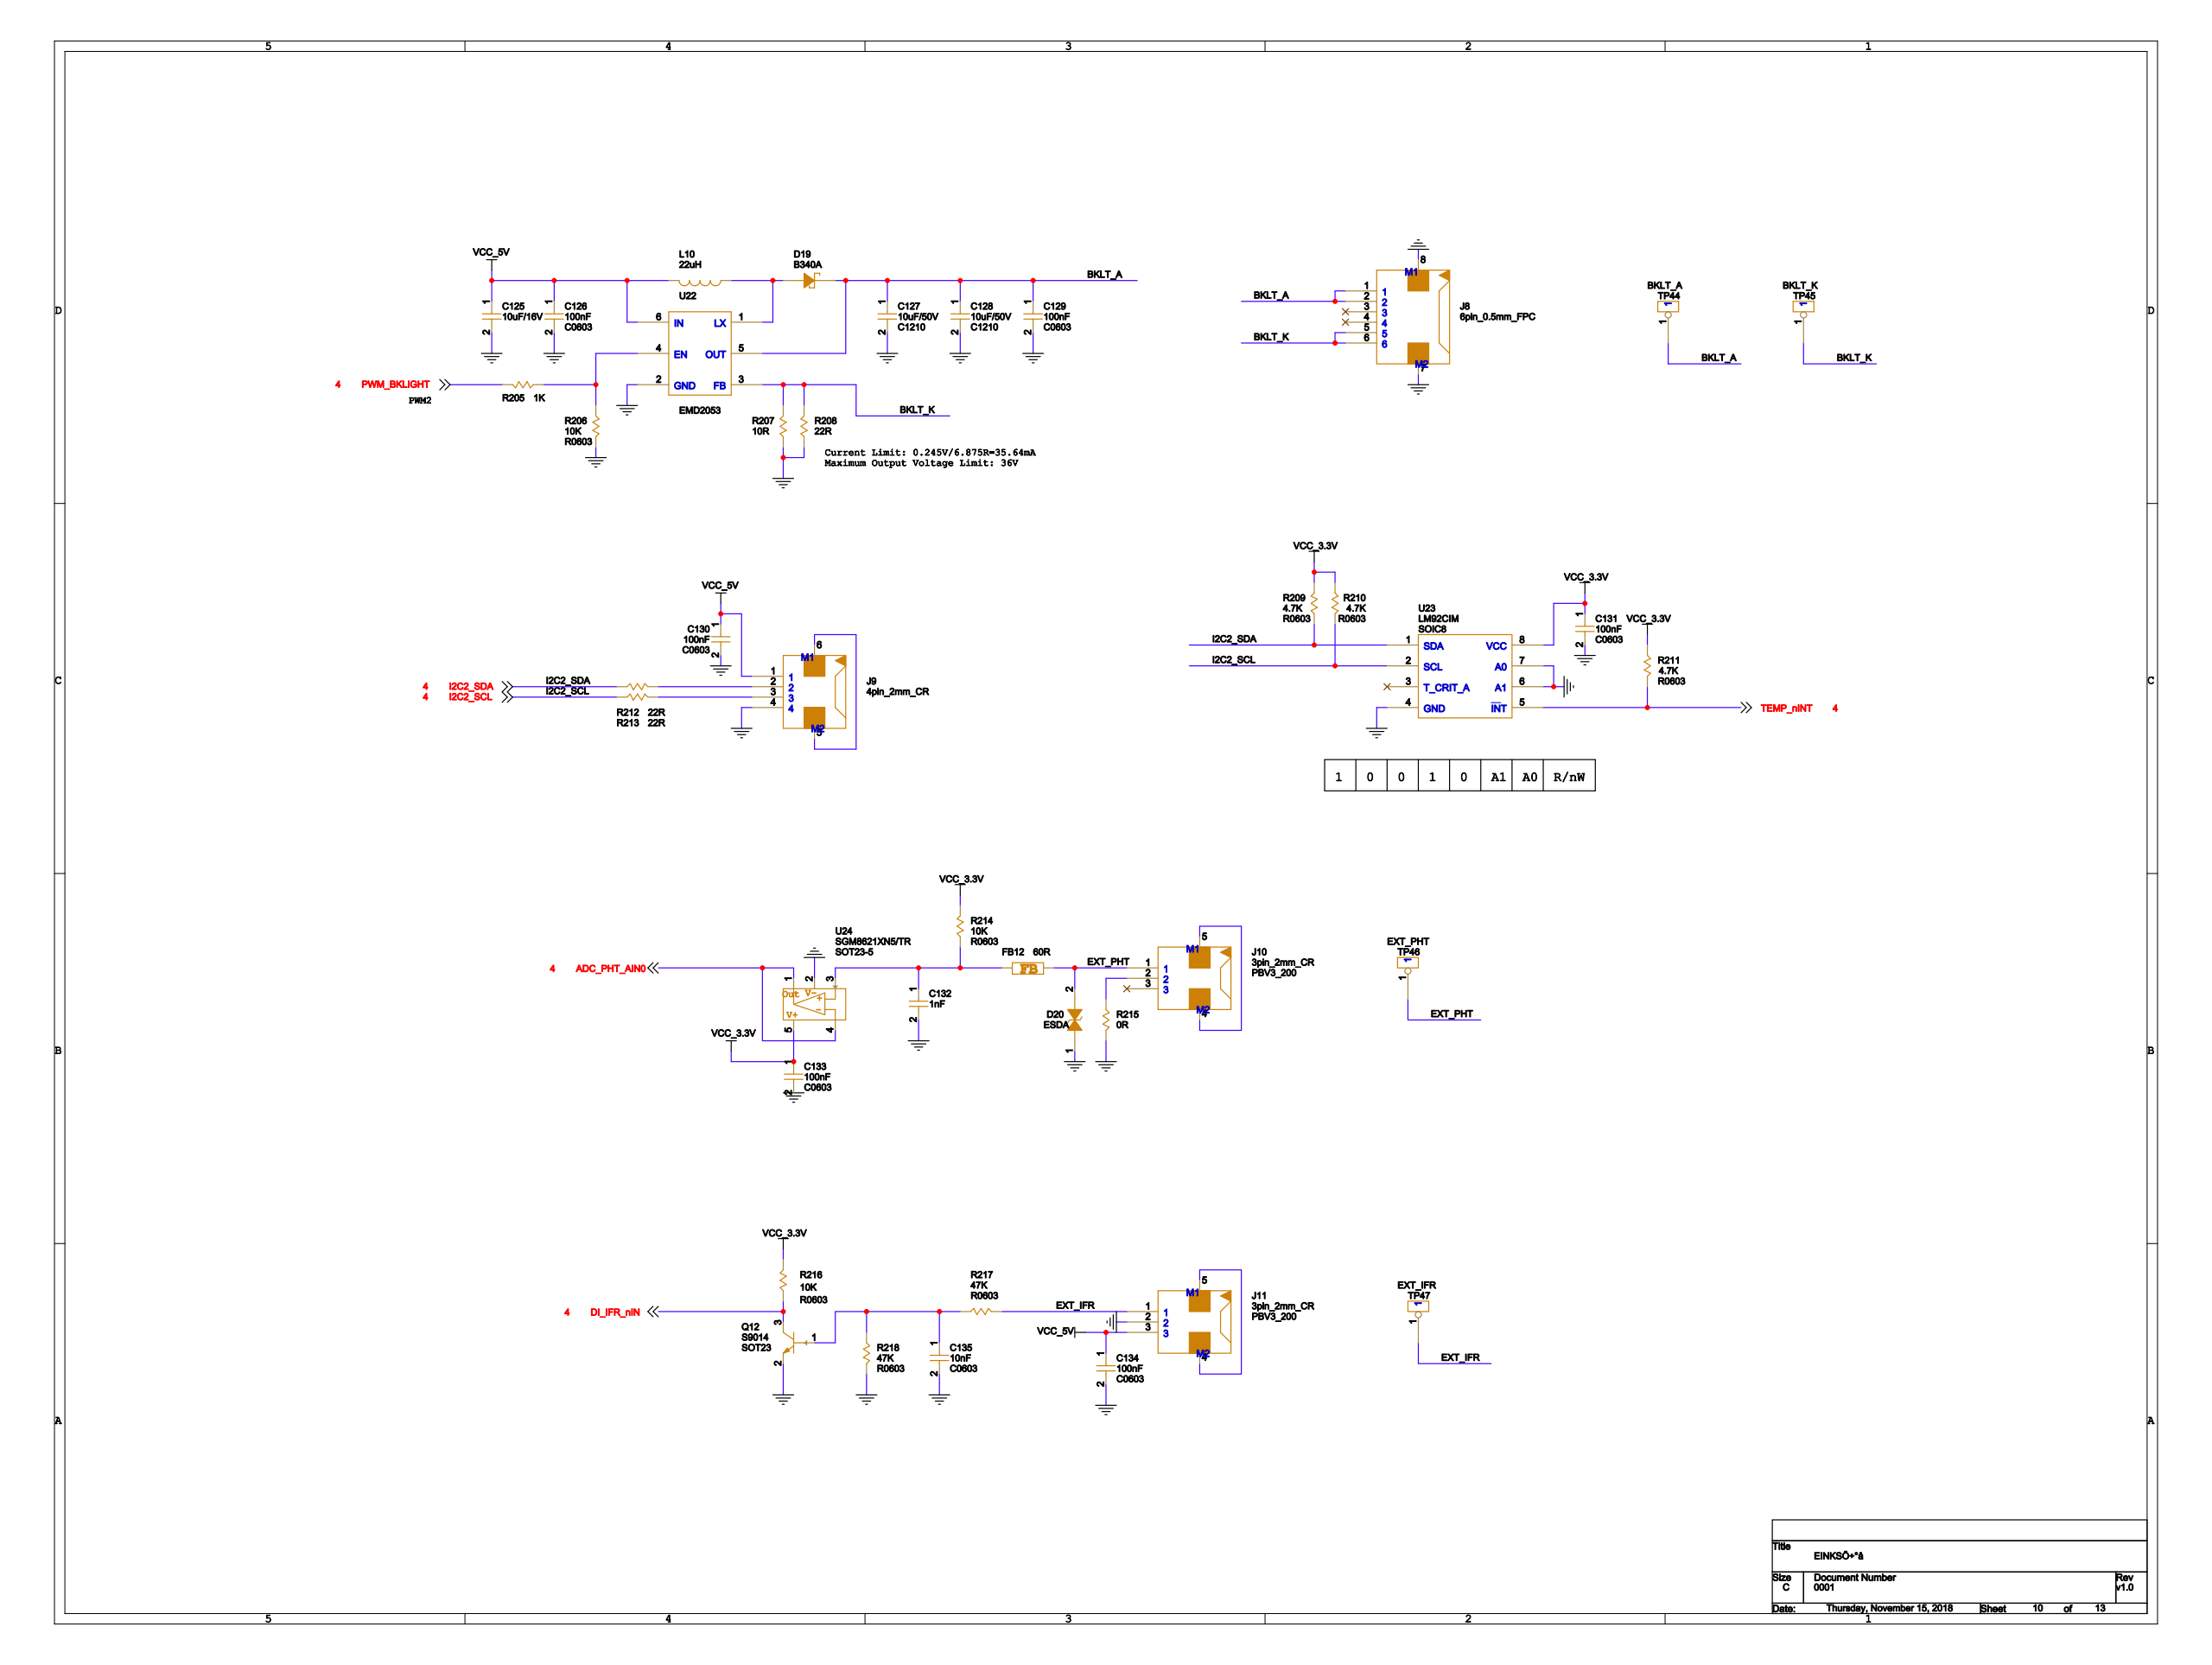Circuit board | Cadence Allegro | 609 parts | 409 nets | one sheet of the schematic
Parts on this sheet (reference | value | footprint):
C125 | 10uF/16V | C1206
C126 | 100nF | C0603
C127 | 10uF/50V | C1210
C128 | 10uF/50V | C1210
C129 | 100nF | C0603
C130 | 100nF | C0603
C131 | 100nF | C0603
C132 | 1nF | C0603
C133 | 100nF | C0603
C134 | 100nF | C0603
C135 | 10nF | C0603
D19 | B340A | DO-214AA
D20 | ESDA | 0603ESDA
FB12 | 60R | FB0603
J8 | 6pin_0.5mm_FPC | 6PIN_05MM_FPC_UP
J9 | 4pin_2mm_CR | PBV4_200
J10 | 3pin_2mm_CR | PBV3_200
J11 | 3pin_2mm_CR | PBV3_200
L10 | 22uH | IND_VLS6045
Q12 | S9014 | SOT23
R205 | 1K | R0603
R206 | 10K | R0603
R207 | 10R | R0603
R208 | 22R | R0603
R209 | 4.7K | R0603
R210 | 4.7K | R0603
R211 | 4.7K | R0603
R212 | 22R | R0603
R213 | 22R | R0603
R214 | 10K | R0603
R215 | 0R | R0603
R216 | 10K | R0603
R217 | 47K | R0603
R218 | 47K | R0603
TP44 | BKLT_A | TP_50
TP45 | BKLT_K | TP_50
TP46 | EXT_PHT | TP_50
TP47 | EXT_IFR | TP_50
U22 | EMD2053 | SOT23-6
U23 | LM92CIM | SOIC8
Nets of these parts (net: part-pin ...):
GND: C125-2 C126-2 C127-2 C128-2 C129-2 C130-2 C131-2 C132-2 C133-2 C134-2 C135-2 D20-1 J8-7 J8-8 J9-4 J11-2 Q12-2 R206-1 R207-2 R208-2 R215-1 R218-2 U22-2 U23-4 U23-6 U23-7
BKLT_A: C127-1 C128-1 C129-1 D19-2 J8-1 J8-2 TP44-1 U22-5
VCC_3.3V: C131-1 C133-1 R209-2 R210-2 R211-2 R214-2 R216-2 U23-8
VCC_5V: C125-1 C126-1 C130-1 C134-1 J9-1 J11-3 L10-2 U22-6
EXT_PHT: D20-2 FB12-2 J10-1 TP46-1
N29143714: C132-1 FB12-1 R214-1
N29143462: J10-2 R215-2
N29143422: J10-4 J10-5
EXT_IFR: J11-1 R217-2 TP47-1
N29145186: J11-4 J11-5
DI_IFR_NIN: Q12-3 R216-1
TEMP_NINT: R211-1 U23-5
I2C2_SCL: R210-1 R213-2 U23-2
I2C2_SDA: R209-1 R212-2 U23-1
PWM_BKLIGHT: R205-2
N29147768: J9-2 R212-1
N29147771: J9-3 R213-1
N29146309: J9-5 J9-6
BKLT_K: J8-5 J8-6 R207-1 R208-1 TP45-1 U22-3
N29109012: R205-1 R206-2 U22-4
N29107844: D19-1 L10-1 U22-1
N29145391: C135-1 Q12-1 R217-1 R218-1